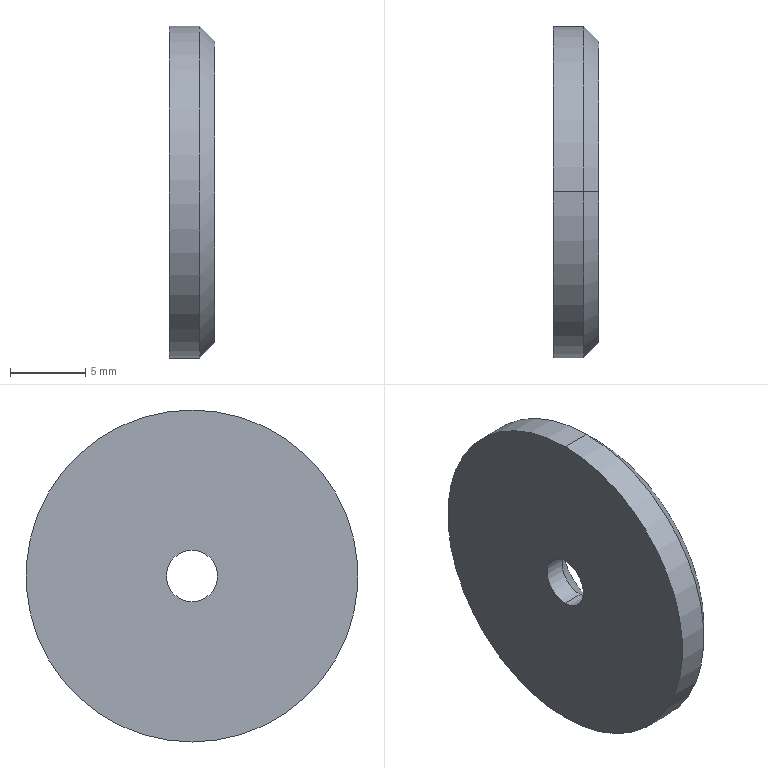Part | STEP file | X77B-01004 | 1 solid | 10 faces | box 3 x 22 x 22 mm | volume 1062 mm3 | cone 4 | cylinder 4 | plane 2 | commonest cylinder face diameters 3.4 x2 22 x2
STEP:
#1=CARTESIAN_POINT('',(-19.981,0.,-10.));
#2=VERTEX_POINT('',#1);
#3=CARTESIAN_POINT('',(-19.981,0.,10.));
#4=VERTEX_POINT('',#3);
#5=CARTESIAN_POINT('',(-19.981,0.,0.));
#6=DIRECTION('',(1.,0.,0.));
#7=DIRECTION('',(0.,0.,-1.));
#8=AXIS2_PLACEMENT_3D('',#5,#6,#7);
#9=CIRCLE('',#8,10.);
#10=EDGE_CURVE('',#2,#4,#9,.T.);
#11=ORIENTED_EDGE('',*,*,#10,.F.);
#12=CARTESIAN_POINT('',(-20.981,0.,-11.));
#13=VERTEX_POINT('',#12);
#14=CARTESIAN_POINT('',(-19.981,0.,-10.));
#15=DIRECTION('',(-0.7071,0.,-0.7071));
#16=VECTOR('',#15,1000.);
#17=LINE('',#14,#16);
#18=EDGE_CURVE('',#2,#13,#17,.T.);
#19=ORIENTED_EDGE('',*,*,#18,.T.);
#20=CARTESIAN_POINT('',(-20.981,0.,11.));
#21=VERTEX_POINT('',#20);
#22=CARTESIAN_POINT('',(-20.981,0.,0.));
#23=DIRECTION('',(-1.,0.,0.));
#24=DIRECTION('',(0.,0.,-1.));
#25=AXIS2_PLACEMENT_3D('',#22,#23,#24);
#26=CIRCLE('',#25,11.);
#27=EDGE_CURVE('',#21,#13,#26,.T.);
#28=ORIENTED_EDGE('',*,*,#27,.F.);
#29=CARTESIAN_POINT('',(-19.981,0.,10.));
#30=DIRECTION('',(-0.7071,0.,0.7071));
#31=VECTOR('',#30,1000.);
#32=LINE('',#29,#31);
#33=EDGE_CURVE('',#4,#21,#32,.T.);
#34=ORIENTED_EDGE('',*,*,#33,.F.);
#35=EDGE_LOOP('',(#11,#19,#28,#34));
#36=FACE_OUTER_BOUND('',#35,.T.);
#37=CARTESIAN_POINT('',(-19.981,0.,0.));
#38=DIRECTION('',(-1.,0.,0.));
#39=DIRECTION('',(0.,0.,1.));
#40=AXIS2_PLACEMENT_3D('',#37,#38,#39);
#41=CONICAL_SURFACE('',#40,10.,0.7854);
#42=ADVANCED_FACE('',(#36),#41,.T.);
#43=CARTESIAN_POINT('',(-21.581,0.,1.7));
#44=VERTEX_POINT('',#43);
#45=CARTESIAN_POINT('',(-21.581,0.,-1.7));
#46=VERTEX_POINT('',#45);
#47=CARTESIAN_POINT('',(-21.581,0.,0.));
#48=DIRECTION('',(1.,0.,0.));
#49=DIRECTION('',(0.,0.,-1.));
#50=AXIS2_PLACEMENT_3D('',#47,#48,#49);
#51=CIRCLE('',#50,1.7);
#52=EDGE_CURVE('',#44,#46,#51,.T.);
#53=ORIENTED_EDGE('',*,*,#52,.F.);
#54=CARTESIAN_POINT('',(-19.981,0.,3.3));
#55=VERTEX_POINT('',#54);
#56=CARTESIAN_POINT('',(-19.981,0.,3.3));
#57=DIRECTION('',(0.7071,0.,0.7071));
#58=VECTOR('',#57,1000.);
#59=LINE('',#56,#58);
#60=EDGE_CURVE('',#44,#55,#59,.T.);
#61=ORIENTED_EDGE('',*,*,#60,.T.);
#62=CARTESIAN_POINT('',(-19.981,0.,-3.3));
#63=VERTEX_POINT('',#62);
#64=CARTESIAN_POINT('',(-19.981,0.,0.));
#65=DIRECTION('',(1.,0.,0.));
#66=DIRECTION('',(0.,0.,-1.));
#67=AXIS2_PLACEMENT_3D('',#64,#65,#66);
#68=CIRCLE('',#67,3.3);
#69=EDGE_CURVE('',#55,#63,#68,.T.);
#70=ORIENTED_EDGE('',*,*,#69,.T.);
#71=CARTESIAN_POINT('',(-19.981,0.,-3.3));
#72=DIRECTION('',(0.7071,0.,-0.7071));
#73=VECTOR('',#72,1000.);
#74=LINE('',#71,#73);
#75=EDGE_CURVE('',#46,#63,#74,.T.);
#76=ORIENTED_EDGE('',*,*,#75,.F.);
#77=EDGE_LOOP('',(#53,#61,#70,#76));
#78=FACE_OUTER_BOUND('',#77,.T.);
#79=CARTESIAN_POINT('',(-19.981,0.,0.));
#80=DIRECTION('',(1.,0.,0.));
#81=DIRECTION('',(0.,0.,-1.));
#82=AXIS2_PLACEMENT_3D('',#79,#80,#81);
#83=CONICAL_SURFACE('',#82,3.3,0.7854);
#84=ADVANCED_FACE('',(#78),#83,.F.);
#85=CARTESIAN_POINT('',(-22.981,0.,1.7));
#86=VERTEX_POINT('',#85);
#87=CARTESIAN_POINT('',(-22.981,0.,-1.7));
#88=VERTEX_POINT('',#87);
#89=CARTESIAN_POINT('',(-22.981,0.,0.));
#90=DIRECTION('',(1.,0.,0.));
#91=DIRECTION('',(0.,0.,-1.));
#92=AXIS2_PLACEMENT_3D('',#89,#90,#91);
#93=CIRCLE('',#92,1.7);
#94=EDGE_CURVE('',#86,#88,#93,.T.);
#95=ORIENTED_EDGE('',*,*,#94,.F.);
#96=CARTESIAN_POINT('',(-19.981,0.,1.7));
#97=DIRECTION('',(1.,0.,0.));
#98=VECTOR('',#97,1000.);
#99=LINE('',#96,#98);
#100=EDGE_CURVE('',#86,#44,#99,.T.);
#101=ORIENTED_EDGE('',*,*,#100,.T.);
#102=ORIENTED_EDGE('',*,*,#52,.T.);
#103=CARTESIAN_POINT('',(-19.981,0.,-1.7));
#104=DIRECTION('',(1.,0.,0.));
#105=VECTOR('',#104,1000.);
#106=LINE('',#103,#105);
#107=EDGE_CURVE('',#88,#46,#106,.T.);
#108=ORIENTED_EDGE('',*,*,#107,.F.);
#109=EDGE_LOOP('',(#95,#101,#102,#108));
#110=FACE_OUTER_BOUND('',#109,.T.);
#111=CARTESIAN_POINT('',(-19.981,0.,0.));
#112=DIRECTION('',(1.,0.,0.));
#113=DIRECTION('',(0.,0.,-1.));
#114=AXIS2_PLACEMENT_3D('',#111,#112,#113);
#115=CYLINDRICAL_SURFACE('',#114,1.7);
#116=ADVANCED_FACE('',(#110),#115,.F.);
#117=CARTESIAN_POINT('',(-22.981,0.,-11.));
#118=VERTEX_POINT('',#117);
#119=CARTESIAN_POINT('',(-22.981,0.,11.));
#120=VERTEX_POINT('',#119);
#121=CARTESIAN_POINT('',(-22.981,0.,0.));
#122=DIRECTION('',(1.,0.,0.));
#123=DIRECTION('',(0.,0.,-1.));
#124=AXIS2_PLACEMENT_3D('',#121,#122,#123);
#125=CIRCLE('',#124,11.);
#126=EDGE_CURVE('',#118,#120,#125,.T.);
#127=ORIENTED_EDGE('',*,*,#126,.T.);
#128=CARTESIAN_POINT('',(0.,0.,11.));
#129=DIRECTION('',(1.,0.,0.));
#130=VECTOR('',#129,1000.);
#131=LINE('',#128,#130);
#132=EDGE_CURVE('',#120,#21,#131,.T.);
#133=ORIENTED_EDGE('',*,*,#132,.T.);
#134=ORIENTED_EDGE('',*,*,#27,.T.);
#135=CARTESIAN_POINT('',(0.,0.,-11.));
#136=DIRECTION('',(1.,0.,0.));
#137=VECTOR('',#136,1000.);
#138=LINE('',#135,#137);
#139=EDGE_CURVE('',#118,#13,#138,.T.);
#140=ORIENTED_EDGE('',*,*,#139,.F.);
#141=EDGE_LOOP('',(#127,#133,#134,#140));
#142=FACE_OUTER_BOUND('',#141,.T.);
#143=CARTESIAN_POINT('',(0.,0.,0.));
#144=DIRECTION('',(1.,0.,0.));
#145=DIRECTION('',(0.,0.,-1.));
#146=AXIS2_PLACEMENT_3D('',#143,#144,#145);
#147=CYLINDRICAL_SURFACE('',#146,11.);
#148=ADVANCED_FACE('',(#142),#147,.T.);
#149=CARTESIAN_POINT('',(-22.981,0.,0.));
#150=DIRECTION('',(1.,0.,0.));
#151=DIRECTION('',(0.,0.,-1.));
#152=AXIS2_PLACEMENT_3D('',#149,#150,#151);
#153=CIRCLE('',#152,1.7);
#154=EDGE_CURVE('',#88,#86,#153,.T.);
#155=ORIENTED_EDGE('',*,*,#154,.T.);
#156=ORIENTED_EDGE('',*,*,#94,.T.);
#157=EDGE_LOOP('',(#155,#156));
#158=FACE_BOUND('',#157,.T.);
#159=ORIENTED_EDGE('',*,*,#126,.F.);
#160=CARTESIAN_POINT('',(-22.981,0.,0.));
#161=DIRECTION('',(1.,0.,0.));
#162=DIRECTION('',(0.,0.,-1.));
#163=AXIS2_PLACEMENT_3D('',#160,#161,#162);
#164=CIRCLE('',#163,11.);
#165=EDGE_CURVE('',#120,#118,#164,.T.);
#166=ORIENTED_EDGE('',*,*,#165,.F.);
#167=EDGE_LOOP('',(#159,#166));
#168=FACE_OUTER_BOUND('',#167,.T.);
#169=CARTESIAN_POINT('',(-22.981,0.,0.));
#170=DIRECTION('',(-1.,0.,0.));
#171=DIRECTION('',(0.,0.,1.));
#172=AXIS2_PLACEMENT_3D('',#169,#170,#171);
#173=PLANE('',#172);
#174=ADVANCED_FACE('',(#158,#168),#173,.T.);
#175=ORIENTED_EDGE('',*,*,#132,.F.);
#176=ORIENTED_EDGE('',*,*,#165,.T.);
#177=ORIENTED_EDGE('',*,*,#139,.T.);
#178=CARTESIAN_POINT('',(-20.981,0.,0.));
#179=DIRECTION('',(-1.,0.,0.));
#180=DIRECTION('',(0.,0.,-1.));
#181=AXIS2_PLACEMENT_3D('',#178,#179,#180);
#182=CIRCLE('',#181,11.);
#183=EDGE_CURVE('',#13,#21,#182,.T.);
#184=ORIENTED_EDGE('',*,*,#183,.T.);
#185=EDGE_LOOP('',(#175,#176,#177,#184));
#186=FACE_OUTER_BOUND('',#185,.T.);
#187=CARTESIAN_POINT('',(0.,0.,0.));
#188=DIRECTION('',(1.,0.,0.));
#189=DIRECTION('',(0.,0.,-1.));
#190=AXIS2_PLACEMENT_3D('',#187,#188,#189);
#191=CYLINDRICAL_SURFACE('',#190,11.);
#192=ADVANCED_FACE('',(#186),#191,.T.);
#193=CARTESIAN_POINT('',(-19.981,0.,0.));
#194=DIRECTION('',(1.,0.,0.));
#195=DIRECTION('',(0.,0.,-1.));
#196=AXIS2_PLACEMENT_3D('',#193,#194,#195);
#197=CIRCLE('',#196,10.);
#198=EDGE_CURVE('',#4,#2,#197,.T.);
#199=ORIENTED_EDGE('',*,*,#198,.T.);
#200=ORIENTED_EDGE('',*,*,#10,.T.);
#201=EDGE_LOOP('',(#199,#200));
#202=FACE_OUTER_BOUND('',#201,.T.);
#203=CARTESIAN_POINT('',(-19.981,0.,0.));
#204=DIRECTION('',(1.,0.,0.));
#205=DIRECTION('',(0.,0.,-1.));
#206=AXIS2_PLACEMENT_3D('',#203,#204,#205);
#207=CIRCLE('',#206,3.3);
#208=EDGE_CURVE('',#63,#55,#207,.T.);
#209=ORIENTED_EDGE('',*,*,#208,.F.);
#210=ORIENTED_EDGE('',*,*,#69,.F.);
#211=EDGE_LOOP('',(#209,#210));
#212=FACE_BOUND('',#211,.T.);
#213=CARTESIAN_POINT('',(-19.981,0.,0.));
#214=DIRECTION('',(1.,0.,0.));
#215=DIRECTION('',(0.,0.,-1.));
#216=AXIS2_PLACEMENT_3D('',#213,#214,#215);
#217=PLANE('',#216);
#218=ADVANCED_FACE('',(#202,#212),#217,.T.);
#219=ORIENTED_EDGE('',*,*,#100,.F.);
#220=ORIENTED_EDGE('',*,*,#154,.F.);
#221=ORIENTED_EDGE('',*,*,#107,.T.);
#222=CARTESIAN_POINT('',(-21.581,0.,0.));
#223=DIRECTION('',(1.,0.,0.));
#224=DIRECTION('',(0.,0.,-1.));
#225=AXIS2_PLACEMENT_3D('',#222,#223,#224);
#226=CIRCLE('',#225,1.7);
#227=EDGE_CURVE('',#46,#44,#226,.T.);
#228=ORIENTED_EDGE('',*,*,#227,.T.);
#229=EDGE_LOOP('',(#219,#220,#221,#228));
#230=FACE_OUTER_BOUND('',#229,.T.);
#231=CARTESIAN_POINT('',(-19.981,0.,0.));
#232=DIRECTION('',(1.,0.,0.));
#233=DIRECTION('',(0.,0.,-1.));
#234=AXIS2_PLACEMENT_3D('',#231,#232,#233);
#235=CYLINDRICAL_SURFACE('',#234,1.7);
#236=ADVANCED_FACE('',(#230),#235,.F.);
#237=ORIENTED_EDGE('',*,*,#60,.F.);
#238=ORIENTED_EDGE('',*,*,#227,.F.);
#239=ORIENTED_EDGE('',*,*,#75,.T.);
#240=ORIENTED_EDGE('',*,*,#208,.T.);
#241=EDGE_LOOP('',(#237,#238,#239,#240));
#242=FACE_OUTER_BOUND('',#241,.T.);
#243=CARTESIAN_POINT('',(-19.981,0.,0.));
#244=DIRECTION('',(1.,0.,0.));
#245=DIRECTION('',(0.,0.,-1.));
#246=AXIS2_PLACEMENT_3D('',#243,#244,#245);
#247=CONICAL_SURFACE('',#246,3.3,0.7854);
#248=ADVANCED_FACE('',(#242),#247,.F.);
#249=ORIENTED_EDGE('',*,*,#18,.F.);
#250=ORIENTED_EDGE('',*,*,#198,.F.);
#251=ORIENTED_EDGE('',*,*,#33,.T.);
#252=ORIENTED_EDGE('',*,*,#183,.F.);
#253=EDGE_LOOP('',(#249,#250,#251,#252));
#254=FACE_OUTER_BOUND('',#253,.T.);
#255=CARTESIAN_POINT('',(-19.981,0.,0.));
#256=DIRECTION('',(-1.,0.,0.));
#257=DIRECTION('',(0.,0.,1.));
#258=AXIS2_PLACEMENT_3D('',#255,#256,#257);
#259=CONICAL_SURFACE('',#258,10.,0.7854);
#260=ADVANCED_FACE('',(#254),#259,.T.);
#261=CLOSED_SHELL('',(#42,#84,#116,#148,#174,#192,#218,#236,#248,#260));
#262=MANIFOLD_SOLID_BREP('',#261);
#263=CARTESIAN_POINT('',(0.,0.,0.));
#264=DIRECTION('',(0.,0.,1.));
#265=DIRECTION('',(1.,0.,0.));
#266=AXIS2_PLACEMENT_3D('',#263,#264,#265);
#267=(LENGTH_UNIT()NAMED_UNIT(*)SI_UNIT(.MILLI.,.METRE.));
#268=UNCERTAINTY_MEASURE_WITH_UNIT(LENGTH_MEASURE(0.00001),#267,'','');
#269=(NAMED_UNIT(*)PLANE_ANGLE_UNIT()SI_UNIT($,.RADIAN.));
#270=(NAMED_UNIT(*)SI_UNIT($,.STERADIAN.)SOLID_ANGLE_UNIT());
#271=(GEOMETRIC_REPRESENTATION_CONTEXT(3)GLOBAL_UNCERTAINTY_ASSIGNED_CONTEXT((#268))GLOBAL_UNIT_ASSIGNED_CONTEXT((#267,#269,#270))REPRESENTATION_CONTEXT('',''));
#272=ADVANCED_BREP_SHAPE_REPRESENTATION('',(#262,#266),#271);